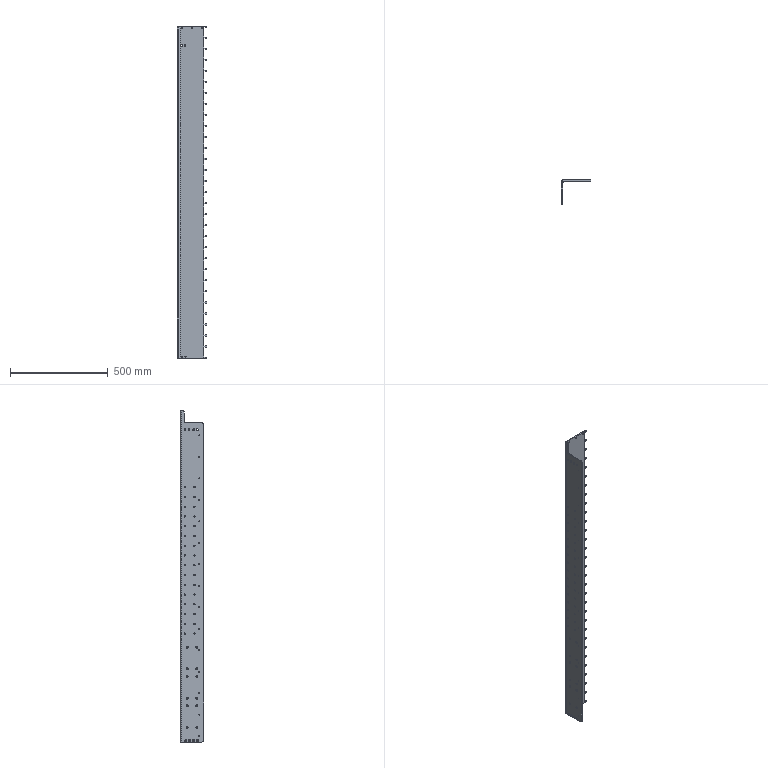Part | SolidWorks | features HoleWzd 10, Fillet 2, LPattern 2, Cut 1, Extrusion 1, ICE 1, MoveFace 1 | 1 solid | 314 faces | box 150 x 120 x 1700 mm | volume 2499600 mm3 | cylinder 160 | plane 142 | cone 12 | commonest cylinder face diameters 6.8 x64 4.2 x36 5.8 x30 10 x24 20 x4 16 x2